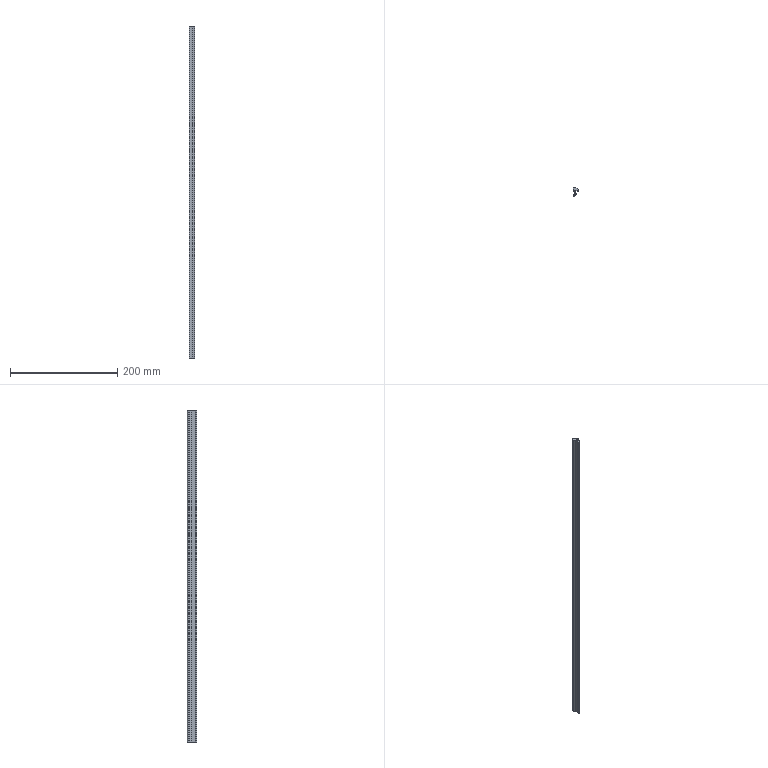Part | SolidWorks | features BaseBody 1, MoveFace 1 | 1 solid | 20 faces | box 10.8 x 17.5 x 620 mm | volume 48856 mm3 | cylinder 11 | plane 9 | commonest cylinder face diameters 1.6 x2 14 x2 0.4 x1 0.6 x1 0.8 x1 2.6 x1
STEP:
#1=CARTESIAN_POINT('',(-3.236,-11.055,520.));
#2=VERTEX_POINT('',#1);
#3=CARTESIAN_POINT('',(-4.3,-10.3,520.));
#4=VERTEX_POINT('',#3);
#5=CARTESIAN_POINT('',(-3.5,-10.3,520.));
#6=DIRECTION('',(0.,0.,-1.));
#7=DIRECTION('',(1.,0.,0.));
#8=AXIS2_PLACEMENT_3D('',#5,#6,#7);
#9=CIRCLE('',#8,0.8);
#10=EDGE_CURVE('',#2,#4,#9,.T.);
#11=ORIENTED_EDGE('',*,*,#10,.T.);
#12=CARTESIAN_POINT('',(-4.3,-10.3,-100.));
#13=VERTEX_POINT('',#12);
#14=CARTESIAN_POINT('',(-4.3,-10.3,-100.));
#15=DIRECTION('',(0.,0.,-1.));
#16=VECTOR('',#15,1000.);
#17=LINE('',#14,#16);
#18=EDGE_CURVE('',#4,#13,#17,.T.);
#19=ORIENTED_EDGE('',*,*,#18,.T.);
#20=CARTESIAN_POINT('',(-3.236,-11.055,-100.));
#21=VERTEX_POINT('',#20);
#22=CARTESIAN_POINT('',(-3.5,-10.3,-100.));
#23=DIRECTION('',(0.,0.,1.));
#24=DIRECTION('',(-1.,0.,0.));
#25=AXIS2_PLACEMENT_3D('',#22,#23,#24);
#26=CIRCLE('',#25,0.8);
#27=EDGE_CURVE('',#13,#21,#26,.T.);
#28=ORIENTED_EDGE('',*,*,#27,.T.);
#29=CARTESIAN_POINT('',(-3.236,-11.055,-100.));
#30=DIRECTION('',(0.,0.,-1.));
#31=VECTOR('',#30,1000.);
#32=LINE('',#29,#31);
#33=EDGE_CURVE('',#2,#21,#32,.T.);
#34=ORIENTED_EDGE('',*,*,#33,.F.);
#35=EDGE_LOOP('',(#11,#19,#28,#34));
#36=FACE_OUTER_BOUND('',#35,.T.);
#37=CARTESIAN_POINT('',(-3.5,-10.3,-100.));
#38=DIRECTION('',(0.,0.,-1.));
#39=DIRECTION('',(-1.,0.,0.));
#40=AXIS2_PLACEMENT_3D('',#37,#38,#39);
#41=CYLINDRICAL_SURFACE('',#40,0.8);
#42=ADVANCED_FACE('',(#36),#41,.T.);
#43=CARTESIAN_POINT('',(1.184,-6.397,-100.));
#44=VERTEX_POINT('',#43);
#45=CARTESIAN_POINT('',(-5.702,-4.29,-100.));
#46=DIRECTION('',(0.,0.,1.));
#47=DIRECTION('',(-1.,0.,0.));
#48=AXIS2_PLACEMENT_3D('',#45,#46,#47);
#49=CIRCLE('',#48,7.201);
#50=EDGE_CURVE('',#21,#44,#49,.T.);
#51=ORIENTED_EDGE('',*,*,#50,.T.);
#52=CARTESIAN_POINT('',(1.184,-6.397,520.));
#53=VERTEX_POINT('',#52);
#54=CARTESIAN_POINT('',(1.184,-6.397,-100.));
#55=DIRECTION('',(0.,0.,1.));
#56=VECTOR('',#55,1000.);
#57=LINE('',#54,#56);
#58=EDGE_CURVE('',#44,#53,#57,.T.);
#59=ORIENTED_EDGE('',*,*,#58,.T.);
#60=CARTESIAN_POINT('',(-5.702,-4.29,520.));
#61=DIRECTION('',(0.,0.,-1.));
#62=DIRECTION('',(1.,0.,0.));
#63=AXIS2_PLACEMENT_3D('',#60,#61,#62);
#64=CIRCLE('',#63,7.201);
#65=EDGE_CURVE('',#53,#2,#64,.T.);
#66=ORIENTED_EDGE('',*,*,#65,.T.);
#67=ORIENTED_EDGE('',*,*,#33,.T.);
#68=EDGE_LOOP('',(#51,#59,#66,#67));
#69=FACE_OUTER_BOUND('',#68,.T.);
#70=CARTESIAN_POINT('',(-5.702,-4.29,-100.));
#71=DIRECTION('',(0.,0.,-1.));
#72=DIRECTION('',(-1.,0.,0.));
#73=AXIS2_PLACEMENT_3D('',#70,#71,#72);
#74=CYLINDRICAL_SURFACE('',#73,7.201);
#75=ADVANCED_FACE('',(#69),#74,.T.);
#76=CARTESIAN_POINT('',(0.9,-6.,-100.));
#77=VERTEX_POINT('',#76);
#78=CARTESIAN_POINT('',(0.9,-6.3,-100.));
#79=DIRECTION('',(0.,0.,1.));
#80=DIRECTION('',(-1.,0.,0.));
#81=AXIS2_PLACEMENT_3D('',#78,#79,#80);
#82=CIRCLE('',#81,0.3);
#83=EDGE_CURVE('',#44,#77,#82,.T.);
#84=ORIENTED_EDGE('',*,*,#83,.T.);
#85=CARTESIAN_POINT('',(0.9,-6.,520.));
#86=VERTEX_POINT('',#85);
#87=CARTESIAN_POINT('',(0.9,-6.,-100.));
#88=DIRECTION('',(0.,0.,1.));
#89=VECTOR('',#88,1000.);
#90=LINE('',#87,#89);
#91=EDGE_CURVE('',#77,#86,#90,.T.);
#92=ORIENTED_EDGE('',*,*,#91,.T.);
#93=CARTESIAN_POINT('',(0.9,-6.3,520.));
#94=DIRECTION('',(0.,0.,-1.));
#95=DIRECTION('',(1.,0.,0.));
#96=AXIS2_PLACEMENT_3D('',#93,#94,#95);
#97=CIRCLE('',#96,0.3);
#98=EDGE_CURVE('',#86,#53,#97,.T.);
#99=ORIENTED_EDGE('',*,*,#98,.T.);
#100=ORIENTED_EDGE('',*,*,#58,.F.);
#101=EDGE_LOOP('',(#84,#92,#99,#100));
#102=FACE_OUTER_BOUND('',#101,.T.);
#103=CARTESIAN_POINT('',(0.9,-6.3,-100.));
#104=DIRECTION('',(0.,0.,-1.));
#105=DIRECTION('',(-1.,0.,0.));
#106=AXIS2_PLACEMENT_3D('',#103,#104,#105);
#107=CYLINDRICAL_SURFACE('',#106,0.3);
#108=ADVANCED_FACE('',(#102),#107,.T.);
#109=CARTESIAN_POINT('',(-2.5,-0.5,-100.));
#110=VERTEX_POINT('',#109);
#111=CARTESIAN_POINT('',(-2.5,-6.153,-100.));
#112=VERTEX_POINT('',#111);
#113=CARTESIAN_POINT('',(-2.5,-6.397,-100.));
#114=DIRECTION('',(0.,-1.,0.));
#115=VECTOR('',#114,1000.);
#116=LINE('',#113,#115);
#117=EDGE_CURVE('',#110,#112,#116,.T.);
#118=ORIENTED_EDGE('',*,*,#117,.F.);
#119=CARTESIAN_POINT('',(-4.2,1.695,-100.));
#120=VERTEX_POINT('',#119);
#121=CARTESIAN_POINT('',(-1.701,1.875,-100.));
#122=DIRECTION('',(0.,0.,1.));
#123=DIRECTION('',(-1.,0.,0.));
#124=AXIS2_PLACEMENT_3D('',#121,#122,#123);
#125=CIRCLE('',#124,2.506);
#126=EDGE_CURVE('',#120,#110,#125,.T.);
#127=ORIENTED_EDGE('',*,*,#126,.F.);
#128=CARTESIAN_POINT('',(-4.2,5.1,-100.));
#129=VERTEX_POINT('',#128);
#130=CARTESIAN_POINT('',(-4.2,-6.397,-100.));
#131=DIRECTION('',(0.,-1.,0.));
#132=VECTOR('',#131,1000.);
#133=LINE('',#130,#132);
#134=EDGE_CURVE('',#129,#120,#133,.T.);
#135=ORIENTED_EDGE('',*,*,#134,.F.);
#136=CARTESIAN_POINT('',(-2.892,6.4,-100.));
#137=VERTEX_POINT('',#136);
#138=CARTESIAN_POINT('',(-2.9,5.1,-100.));
#139=DIRECTION('',(0.,0.,1.));
#140=DIRECTION('',(-1.,0.,0.));
#141=AXIS2_PLACEMENT_3D('',#138,#139,#140);
#142=CIRCLE('',#141,1.3);
#143=EDGE_CURVE('',#137,#129,#142,.T.);
#144=ORIENTED_EDGE('',*,*,#143,.F.);
#145=CARTESIAN_POINT('',(0.5,5.5,-100.));
#146=VERTEX_POINT('',#145);
#147=CARTESIAN_POINT('',(-2.934,-0.5999,-100.));
#148=DIRECTION('',(0.,0.,1.));
#149=DIRECTION('',(-1.,0.,0.));
#150=AXIS2_PLACEMENT_3D('',#147,#148,#149);
#151=CIRCLE('',#150,7.);
#152=EDGE_CURVE('',#146,#137,#151,.T.);
#153=ORIENTED_EDGE('',*,*,#152,.F.);
#154=CARTESIAN_POINT('',(5.5,1.7,-100.));
#155=VERTEX_POINT('',#154);
#156=CARTESIAN_POINT('',(5.5,1.7,-100.));
#157=DIRECTION('',(-0.7962,0.6051,0.));
#158=VECTOR('',#157,1000.);
#159=LINE('',#156,#158);
#160=EDGE_CURVE('',#155,#146,#159,.T.);
#161=ORIENTED_EDGE('',*,*,#160,.F.);
#162=CARTESIAN_POINT('',(6.458,-0.2215,-100.));
#163=VERTEX_POINT('',#162);
#164=CARTESIAN_POINT('',(6.458,-0.2215,-100.));
#165=DIRECTION('',(-0.4462,0.8949,0.));
#166=VECTOR('',#165,1000.);
#167=LINE('',#164,#166);
#168=EDGE_CURVE('',#163,#155,#167,.T.);
#169=ORIENTED_EDGE('',*,*,#168,.F.);
#170=CARTESIAN_POINT('',(5.895,-0.7433,-100.));
#171=VERTEX_POINT('',#170);
#172=CARTESIAN_POINT('',(6.1,-0.4,-100.));
#173=DIRECTION('',(0.,0.,1.));
#174=DIRECTION('',(-1.,0.,0.));
#175=AXIS2_PLACEMENT_3D('',#172,#173,#174);
#176=CIRCLE('',#175,0.4);
#177=EDGE_CURVE('',#171,#163,#176,.T.);
#178=ORIENTED_EDGE('',*,*,#177,.F.);
#179=CARTESIAN_POINT('',(3.,0.,-100.));
#180=VERTEX_POINT('',#179);
#181=CARTESIAN_POINT('',(2.746,-6.995,-100.));
#182=DIRECTION('',(0.,0.,-1.));
#183=DIRECTION('',(-1.,0.,0.));
#184=AXIS2_PLACEMENT_3D('',#181,#182,#183);
#185=CIRCLE('',#184,7.);
#186=EDGE_CURVE('',#180,#171,#185,.T.);
#187=ORIENTED_EDGE('',*,*,#186,.F.);
#188=CARTESIAN_POINT('',(0.,0.,-100.));
#189=VERTEX_POINT('',#188);
#190=CARTESIAN_POINT('',(-6.814,0.,-100.));
#191=DIRECTION('',(1.,0.,0.));
#192=VECTOR('',#191,1000.);
#193=LINE('',#190,#192);
#194=EDGE_CURVE('',#189,#180,#193,.T.);
#195=ORIENTED_EDGE('',*,*,#194,.F.);
#196=CARTESIAN_POINT('',(0.,-5.8,-100.));
#197=VERTEX_POINT('',#196);
#198=CARTESIAN_POINT('',(0.,-6.397,-100.));
#199=DIRECTION('',(0.,1.,0.));
#200=VECTOR('',#199,1000.);
#201=LINE('',#198,#200);
#202=EDGE_CURVE('',#197,#189,#201,.T.);
#203=ORIENTED_EDGE('',*,*,#202,.F.);
#204=CARTESIAN_POINT('',(0.2,-6.,-100.));
#205=VERTEX_POINT('',#204);
#206=CARTESIAN_POINT('',(0.2,-5.8,-100.));
#207=DIRECTION('',(0.,0.,1.));
#208=DIRECTION('',(-1.,0.,0.));
#209=AXIS2_PLACEMENT_3D('',#206,#207,#208);
#210=CIRCLE('',#209,0.2);
#211=EDGE_CURVE('',#197,#205,#210,.T.);
#212=ORIENTED_EDGE('',*,*,#211,.T.);
#213=CARTESIAN_POINT('',(-6.814,-6.,-100.));
#214=DIRECTION('',(-1.,0.,0.));
#215=VECTOR('',#214,1000.);
#216=LINE('',#213,#215);
#217=EDGE_CURVE('',#77,#205,#216,.T.);
#218=ORIENTED_EDGE('',*,*,#217,.F.);
#219=ORIENTED_EDGE('',*,*,#83,.F.);
#220=ORIENTED_EDGE('',*,*,#50,.F.);
#221=ORIENTED_EDGE('',*,*,#27,.F.);
#222=CARTESIAN_POINT('',(-3.998,-9.674,-100.));
#223=VERTEX_POINT('',#222);
#224=CARTESIAN_POINT('',(-3.5,-10.3,-100.));
#225=DIRECTION('',(0.,0.,1.));
#226=DIRECTION('',(-1.,0.,0.));
#227=AXIS2_PLACEMENT_3D('',#224,#225,#226);
#228=CIRCLE('',#227,0.8);
#229=EDGE_CURVE('',#223,#13,#228,.T.);
#230=ORIENTED_EDGE('',*,*,#229,.F.);
#231=CARTESIAN_POINT('',(-6.814,-6.397,-100.));
#232=DIRECTION('',(0.,0.,-1.));
#233=DIRECTION('',(-1.,0.,0.));
#234=AXIS2_PLACEMENT_3D('',#231,#232,#233);
#235=CIRCLE('',#234,4.321);
#236=EDGE_CURVE('',#112,#223,#235,.T.);
#237=ORIENTED_EDGE('',*,*,#236,.F.);
#238=EDGE_LOOP('',(#118,#127,#135,#144,#153,#161,#169,#178,#187,#195,#203,#212,#218,#219,#220,#221,#230,#237));
#239=FACE_OUTER_BOUND('',#238,.T.);
#240=CARTESIAN_POINT('',(-6.814,-6.397,-100.));
#241=DIRECTION('',(0.,0.,1.));
#242=DIRECTION('',(1.,0.,0.));
#243=AXIS2_PLACEMENT_3D('',#240,#241,#242);
#244=PLANE('',#243);
#245=ADVANCED_FACE('',(#239),#244,.F.);
#246=ORIENTED_EDGE('',*,*,#18,.F.);
#247=CARTESIAN_POINT('',(-3.998,-9.674,520.));
#248=VERTEX_POINT('',#247);
#249=CARTESIAN_POINT('',(-3.5,-10.3,520.));
#250=DIRECTION('',(0.,0.,-1.));
#251=DIRECTION('',(1.,0.,0.));
#252=AXIS2_PLACEMENT_3D('',#249,#250,#251);
#253=CIRCLE('',#252,0.8);
#254=EDGE_CURVE('',#4,#248,#253,.T.);
#255=ORIENTED_EDGE('',*,*,#254,.T.);
#256=CARTESIAN_POINT('',(-3.998,-9.674,-100.));
#257=DIRECTION('',(0.,0.,-1.));
#258=VECTOR('',#257,1000.);
#259=LINE('',#256,#258);
#260=EDGE_CURVE('',#248,#223,#259,.T.);
#261=ORIENTED_EDGE('',*,*,#260,.T.);
#262=ORIENTED_EDGE('',*,*,#229,.T.);
#263=EDGE_LOOP('',(#246,#255,#261,#262));
#264=FACE_OUTER_BOUND('',#263,.T.);
#265=CARTESIAN_POINT('',(-3.5,-10.3,-100.));
#266=DIRECTION('',(0.,0.,-1.));
#267=DIRECTION('',(-1.,0.,0.));
#268=AXIS2_PLACEMENT_3D('',#265,#266,#267);
#269=CYLINDRICAL_SURFACE('',#268,0.8);
#270=ADVANCED_FACE('',(#264),#269,.T.);
#271=CARTESIAN_POINT('',(-4.2,1.695,520.));
#272=VERTEX_POINT('',#271);
#273=CARTESIAN_POINT('',(-2.5,-0.5,520.));
#274=VERTEX_POINT('',#273);
#275=CARTESIAN_POINT('',(-1.701,1.875,520.));
#276=DIRECTION('',(0.,0.,1.));
#277=DIRECTION('',(1.,0.,0.));
#278=AXIS2_PLACEMENT_3D('',#275,#276,#277);
#279=CIRCLE('',#278,2.506);
#280=EDGE_CURVE('',#272,#274,#279,.T.);
#281=ORIENTED_EDGE('',*,*,#280,.T.);
#282=CARTESIAN_POINT('',(-2.5,-6.153,520.));
#283=VERTEX_POINT('',#282);
#284=CARTESIAN_POINT('',(-2.5,-6.397,520.));
#285=DIRECTION('',(0.,-1.,0.));
#286=VECTOR('',#285,1000.);
#287=LINE('',#284,#286);
#288=EDGE_CURVE('',#274,#283,#287,.T.);
#289=ORIENTED_EDGE('',*,*,#288,.T.);
#290=CARTESIAN_POINT('',(-6.814,-6.397,520.));
#291=DIRECTION('',(0.,0.,-1.));
#292=DIRECTION('',(1.,0.,0.));
#293=AXIS2_PLACEMENT_3D('',#290,#291,#292);
#294=CIRCLE('',#293,4.321);
#295=EDGE_CURVE('',#283,#248,#294,.T.);
#296=ORIENTED_EDGE('',*,*,#295,.T.);
#297=ORIENTED_EDGE('',*,*,#254,.F.);
#298=ORIENTED_EDGE('',*,*,#10,.F.);
#299=ORIENTED_EDGE('',*,*,#65,.F.);
#300=ORIENTED_EDGE('',*,*,#98,.F.);
#301=CARTESIAN_POINT('',(0.2,-6.,520.));
#302=VERTEX_POINT('',#301);
#303=CARTESIAN_POINT('',(-6.814,-6.,520.));
#304=DIRECTION('',(-1.,0.,0.));
#305=VECTOR('',#304,1000.);
#306=LINE('',#303,#305);
#307=EDGE_CURVE('',#86,#302,#306,.T.);
#308=ORIENTED_EDGE('',*,*,#307,.T.);
#309=CARTESIAN_POINT('',(0.,-5.8,520.));
#310=VERTEX_POINT('',#309);
#311=CARTESIAN_POINT('',(0.2,-5.8,520.));
#312=DIRECTION('',(0.,0.,-1.));
#313=DIRECTION('',(1.,0.,0.));
#314=AXIS2_PLACEMENT_3D('',#311,#312,#313);
#315=CIRCLE('',#314,0.2);
#316=EDGE_CURVE('',#302,#310,#315,.T.);
#317=ORIENTED_EDGE('',*,*,#316,.T.);
#318=CARTESIAN_POINT('',(0.,0.,520.));
#319=VERTEX_POINT('',#318);
#320=CARTESIAN_POINT('',(0.,-6.397,520.));
#321=DIRECTION('',(0.,1.,0.));
#322=VECTOR('',#321,1000.);
#323=LINE('',#320,#322);
#324=EDGE_CURVE('',#310,#319,#323,.T.);
#325=ORIENTED_EDGE('',*,*,#324,.T.);
#326=CARTESIAN_POINT('',(3.,0.,520.));
#327=VERTEX_POINT('',#326);
#328=CARTESIAN_POINT('',(-6.814,0.,520.));
#329=DIRECTION('',(1.,0.,0.));
#330=VECTOR('',#329,1000.);
#331=LINE('',#328,#330);
#332=EDGE_CURVE('',#319,#327,#331,.T.);
#333=ORIENTED_EDGE('',*,*,#332,.T.);
#334=CARTESIAN_POINT('',(5.895,-0.7433,520.));
#335=VERTEX_POINT('',#334);
#336=CARTESIAN_POINT('',(2.746,-6.995,520.));
#337=DIRECTION('',(0.,0.,-1.));
#338=DIRECTION('',(1.,0.,0.));
#339=AXIS2_PLACEMENT_3D('',#336,#337,#338);
#340=CIRCLE('',#339,7.);
#341=EDGE_CURVE('',#327,#335,#340,.T.);
#342=ORIENTED_EDGE('',*,*,#341,.T.);
#343=CARTESIAN_POINT('',(6.458,-0.2215,520.));
#344=VERTEX_POINT('',#343);
#345=CARTESIAN_POINT('',(6.1,-0.4,520.));
#346=DIRECTION('',(0.,0.,-1.));
#347=DIRECTION('',(1.,0.,0.));
#348=AXIS2_PLACEMENT_3D('',#345,#346,#347);
#349=CIRCLE('',#348,0.4);
#350=EDGE_CURVE('',#344,#335,#349,.T.);
#351=ORIENTED_EDGE('',*,*,#350,.F.);
#352=CARTESIAN_POINT('',(5.5,1.7,520.));
#353=VERTEX_POINT('',#352);
#354=CARTESIAN_POINT('',(6.282,0.1323,520.));
#355=DIRECTION('',(-0.4462,0.8949,0.));
#356=VECTOR('',#355,1000.);
#357=LINE('',#354,#356);
#358=EDGE_CURVE('',#344,#353,#357,.T.);
#359=ORIENTED_EDGE('',*,*,#358,.T.);
#360=CARTESIAN_POINT('',(0.5,5.5,520.));
#361=VERTEX_POINT('',#360);
#362=CARTESIAN_POINT('',(1.595,4.668,520.));
#363=DIRECTION('',(-0.7962,0.6051,0.));
#364=VECTOR('',#363,1000.);
#365=LINE('',#362,#364);
#366=EDGE_CURVE('',#353,#361,#365,.T.);
#367=ORIENTED_EDGE('',*,*,#366,.T.);
#368=CARTESIAN_POINT('',(-2.892,6.4,520.));
#369=VERTEX_POINT('',#368);
#370=CARTESIAN_POINT('',(-2.934,-0.5999,520.));
#371=DIRECTION('',(0.,0.,1.));
#372=DIRECTION('',(1.,0.,0.));
#373=AXIS2_PLACEMENT_3D('',#370,#371,#372);
#374=CIRCLE('',#373,7.);
#375=EDGE_CURVE('',#361,#369,#374,.T.);
#376=ORIENTED_EDGE('',*,*,#375,.T.);
#377=CARTESIAN_POINT('',(-4.2,5.1,520.));
#378=VERTEX_POINT('',#377);
#379=CARTESIAN_POINT('',(-2.9,5.1,520.));
#380=DIRECTION('',(0.,0.,1.));
#381=DIRECTION('',(1.,0.,0.));
#382=AXIS2_PLACEMENT_3D('',#379,#380,#381);
#383=CIRCLE('',#382,1.3);
#384=EDGE_CURVE('',#369,#378,#383,.T.);
#385=ORIENTED_EDGE('',*,*,#384,.T.);
#386=CARTESIAN_POINT('',(-4.2,-6.397,520.));
#387=DIRECTION('',(0.,-1.,0.));
#388=VECTOR('',#387,1000.);
#389=LINE('',#386,#388);
#390=EDGE_CURVE('',#378,#272,#389,.T.);
#391=ORIENTED_EDGE('',*,*,#390,.T.);
#392=EDGE_LOOP('',(#281,#289,#296,#297,#298,#299,#300,#308,#317,#325,#333,#342,#351,#359,#367,#376,#385,#391));
#393=FACE_OUTER_BOUND('',#392,.T.);
#394=CARTESIAN_POINT('',(-6.814,-6.397,520.));
#395=DIRECTION('',(0.,0.,1.));
#396=DIRECTION('',(1.,0.,0.));
#397=AXIS2_PLACEMENT_3D('',#394,#395,#396);
#398=PLANE('',#397);
#399=ADVANCED_FACE('',(#393),#398,.T.);
#400=ORIENTED_EDGE('',*,*,#217,.T.);
#401=CARTESIAN_POINT('',(0.2,-6.,-100.));
#402=DIRECTION('',(0.,0.,1.));
#403=VECTOR('',#402,1000.);
#404=LINE('',#401,#403);
#405=EDGE_CURVE('',#205,#302,#404,.T.);
#406=ORIENTED_EDGE('',*,*,#405,.T.);
#407=ORIENTED_EDGE('',*,*,#307,.F.);
#408=ORIENTED_EDGE('',*,*,#91,.F.);
#409=EDGE_LOOP('',(#400,#406,#407,#408));
#410=FACE_OUTER_BOUND('',#409,.T.);
#411=CARTESIAN_POINT('',(0.9,-6.,-100.));
#412=DIRECTION('',(0.,1.,0.));
#413=DIRECTION('',(0.,0.,1.));
#414=AXIS2_PLACEMENT_3D('',#411,#412,#413);
#415=PLANE('',#414);
#416=ADVANCED_FACE('',(#410),#415,.T.);
#417=CARTESIAN_POINT('',(-2.5,-6.153,-100.));
#418=DIRECTION('',(0.,0.,1.));
#419=VECTOR('',#418,1000.);
#420=LINE('',#417,#419);
#421=EDGE_CURVE('',#112,#283,#420,.T.);
#422=ORIENTED_EDGE('',*,*,#421,.F.);
#423=ORIENTED_EDGE('',*,*,#236,.T.);
#424=ORIENTED_EDGE('',*,*,#260,.F.);
#425=ORIENTED_EDGE('',*,*,#295,.F.);
#426=EDGE_LOOP('',(#422,#423,#424,#425));
#427=FACE_OUTER_BOUND('',#426,.T.);
#428=CARTESIAN_POINT('',(-6.814,-6.397,-100.));
#429=DIRECTION('',(0.,0.,-1.));
#430=DIRECTION('',(-1.,0.,0.));
#431=AXIS2_PLACEMENT_3D('',#428,#429,#430);
#432=CYLINDRICAL_SURFACE('',#431,4.321);
#433=ADVANCED_FACE('',(#427),#432,.F.);
#434=ORIENTED_EDGE('',*,*,#117,.T.);
#435=ORIENTED_EDGE('',*,*,#421,.T.);
#436=ORIENTED_EDGE('',*,*,#288,.F.);
#437=CARTESIAN_POINT('',(-2.5,-0.5,-100.));
#438=DIRECTION('',(0.,0.,-1.));
#439=VECTOR('',#438,1000.);
#440=LINE('',#437,#439);
#441=EDGE_CURVE('',#274,#110,#440,.T.);
#442=ORIENTED_EDGE('',*,*,#441,.T.);
#443=EDGE_LOOP('',(#434,#435,#436,#442));
#444=FACE_OUTER_BOUND('',#443,.T.);
#445=CARTESIAN_POINT('',(-2.5,-0.5,-100.));
#446=DIRECTION('',(-1.,0.,0.));
#447=DIRECTION('',(0.,0.,1.));
#448=AXIS2_PLACEMENT_3D('',#445,#446,#447);
#449=PLANE('',#448);
#450=ADVANCED_FACE('',(#444),#449,.T.);
#451=ORIENTED_EDGE('',*,*,#126,.T.);
#452=ORIENTED_EDGE('',*,*,#441,.F.);
#453=ORIENTED_EDGE('',*,*,#280,.F.);
#454=CARTESIAN_POINT('',(-4.2,1.695,-100.));
#455=DIRECTION('',(0.,0.,-1.));
#456=VECTOR('',#455,1000.);
#457=LINE('',#454,#456);
#458=EDGE_CURVE('',#272,#120,#457,.T.);
#459=ORIENTED_EDGE('',*,*,#458,.T.);
#460=EDGE_LOOP('',(#451,#452,#453,#459));
#461=FACE_OUTER_BOUND('',#460,.T.);
#462=CARTESIAN_POINT('',(-1.701,1.875,-100.));
#463=DIRECTION('',(0.,0.,-1.));
#464=DIRECTION('',(-1.,0.,0.));
#465=AXIS2_PLACEMENT_3D('',#462,#463,#464);
#466=CYLINDRICAL_SURFACE('',#465,2.506);
#467=ADVANCED_FACE('',(#461),#466,.T.);
#468=ORIENTED_EDGE('',*,*,#134,.T.);
#469=ORIENTED_EDGE('',*,*,#458,.F.);
#470=ORIENTED_EDGE('',*,*,#390,.F.);
#471=CARTESIAN_POINT('',(-4.2,5.1,-100.));
#472=DIRECTION('',(0.,0.,-1.));
#473=VECTOR('',#472,1000.);
#474=LINE('',#471,#473);
#475=EDGE_CURVE('',#378,#129,#474,.T.);
#476=ORIENTED_EDGE('',*,*,#475,.T.);
#477=EDGE_LOOP('',(#468,#469,#470,#476));
#478=FACE_OUTER_BOUND('',#477,.T.);
#479=CARTESIAN_POINT('',(-4.2,5.1,-100.));
#480=DIRECTION('',(-1.,0.,0.));
#481=DIRECTION('',(0.,0.,1.));
#482=AXIS2_PLACEMENT_3D('',#479,#480,#481);
#483=PLANE('',#482);
#484=ADVANCED_FACE('',(#478),#483,.T.);
#485=ORIENTED_EDGE('',*,*,#143,.T.);
#486=ORIENTED_EDGE('',*,*,#475,.F.);
#487=ORIENTED_EDGE('',*,*,#384,.F.);
#488=CARTESIAN_POINT('',(-2.892,6.4,-100.));
#489=DIRECTION('',(0.,0.,-1.));
#490=VECTOR('',#489,1000.);
#491=LINE('',#488,#490);
#492=EDGE_CURVE('',#369,#137,#491,.T.);
#493=ORIENTED_EDGE('',*,*,#492,.T.);
#494=EDGE_LOOP('',(#485,#486,#487,#493));
#495=FACE_OUTER_BOUND('',#494,.T.);
#496=CARTESIAN_POINT('',(-2.9,5.1,-100.));
#497=DIRECTION('',(0.,0.,-1.));
#498=DIRECTION('',(-1.,0.,0.));
#499=AXIS2_PLACEMENT_3D('',#496,#497,#498);
#500=CYLINDRICAL_SURFACE('',#499,1.3);
#501=ADVANCED_FACE('',(#495),#500,.T.);
#502=ORIENTED_EDGE('',*,*,#152,.T.);
#503=ORIENTED_EDGE('',*,*,#492,.F.);
#504=ORIENTED_EDGE('',*,*,#375,.F.);
#505=CARTESIAN_POINT('',(0.5,5.5,-100.));
#506=DIRECTION('',(0.,0.,-1.));
#507=VECTOR('',#506,1000.);
#508=LINE('',#505,#507);
#509=EDGE_CURVE('',#361,#146,#508,.T.);
#510=ORIENTED_EDGE('',*,*,#509,.T.);
#511=EDGE_LOOP('',(#502,#503,#504,#510));
#512=FACE_OUTER_BOUND('',#511,.T.);
#513=CARTESIAN_POINT('',(-2.934,-0.5999,-100.));
#514=DIRECTION('',(0.,0.,-1.));
#515=DIRECTION('',(-1.,0.,0.));
#516=AXIS2_PLACEMENT_3D('',#513,#514,#515);
#517=CYLINDRICAL_SURFACE('',#516,7.);
#518=ADVANCED_FACE('',(#512),#517,.T.);
#519=ORIENTED_EDGE('',*,*,#160,.T.);
#520=ORIENTED_EDGE('',*,*,#509,.F.);
#521=ORIENTED_EDGE('',*,*,#366,.F.);
#522=CARTESIAN_POINT('',(5.5,1.7,-100.));
#523=DIRECTION('',(0.,0.,-1.));
#524=VECTOR('',#523,1000.);
#525=LINE('',#522,#524);
#526=EDGE_CURVE('',#353,#155,#525,.T.);
#527=ORIENTED_EDGE('',*,*,#526,.T.);
#528=EDGE_LOOP('',(#519,#520,#521,#527));
#529=FACE_OUTER_BOUND('',#528,.T.);
#530=CARTESIAN_POINT('',(5.5,1.7,-100.));
#531=DIRECTION('',(0.6051,0.7962,0.));
#532=DIRECTION('',(-0.7962,0.6051,0.));
#533=AXIS2_PLACEMENT_3D('',#530,#531,#532);
#534=PLANE('',#533);
#535=ADVANCED_FACE('',(#529),#534,.T.);
#536=ORIENTED_EDGE('',*,*,#168,.T.);
#537=ORIENTED_EDGE('',*,*,#526,.F.);
#538=ORIENTED_EDGE('',*,*,#358,.F.);
#539=CARTESIAN_POINT('',(6.458,-0.2215,-100.));
#540=DIRECTION('',(0.,0.,-1.));
#541=VECTOR('',#540,1000.);
#542=LINE('',#539,#541);
#543=EDGE_CURVE('',#344,#163,#542,.T.);
#544=ORIENTED_EDGE('',*,*,#543,.T.);
#545=EDGE_LOOP('',(#536,#537,#538,#544));
#546=FACE_OUTER_BOUND('',#545,.T.);
#547=CARTESIAN_POINT('',(6.458,-0.2215,-100.));
#548=DIRECTION('',(0.8949,0.4462,0.));
#549=DIRECTION('',(-0.4462,0.8949,0.));
#550=AXIS2_PLACEMENT_3D('',#547,#548,#549);
#551=PLANE('',#550);
#552=ADVANCED_FACE('',(#546),#551,.T.);
#553=CARTESIAN_POINT('',(3.,0.,-100.));
#554=DIRECTION('',(0.,0.,1.));
#555=VECTOR('',#554,1000.);
#556=LINE('',#553,#555);
#557=EDGE_CURVE('',#180,#327,#556,.T.);
#558=ORIENTED_EDGE('',*,*,#557,.F.);
#559=ORIENTED_EDGE('',*,*,#186,.T.);
#560=CARTESIAN_POINT('',(5.895,-0.7433,-100.));
#561=DIRECTION('',(0.,0.,-1.));
#562=VECTOR('',#561,1000.);
#563=LINE('',#560,#562);
#564=EDGE_CURVE('',#335,#171,#563,.T.);
#565=ORIENTED_EDGE('',*,*,#564,.F.);
#566=ORIENTED_EDGE('',*,*,#341,.F.);
#567=EDGE_LOOP('',(#558,#559,#565,#566));
#568=FACE_OUTER_BOUND('',#567,.T.);
#569=CARTESIAN_POINT('',(2.746,-6.995,-100.));
#570=DIRECTION('',(0.,0.,-1.));
#571=DIRECTION('',(-1.,0.,0.));
#572=AXIS2_PLACEMENT_3D('',#569,#570,#571);
#573=CYLINDRICAL_SURFACE('',#572,7.);
#574=ADVANCED_FACE('',(#568),#573,.F.);
#575=ORIENTED_EDGE('',*,*,#194,.T.);
#576=ORIENTED_EDGE('',*,*,#557,.T.);
#577=ORIENTED_EDGE('',*,*,#332,.F.);
#578=CARTESIAN_POINT('',(0.,0.,-100.));
#579=DIRECTION('',(0.,0.,-1.));
#580=VECTOR('',#579,1000.);
#581=LINE('',#578,#580);
#582=EDGE_CURVE('',#319,#189,#581,.T.);
#583=ORIENTED_EDGE('',*,*,#582,.T.);
#584=EDGE_LOOP('',(#575,#576,#577,#583));
#585=FACE_OUTER_BOUND('',#584,.T.);
#586=CARTESIAN_POINT('',(0.,0.,-100.));
#587=DIRECTION('',(0.,-1.,0.));
#588=DIRECTION('',(0.,0.,-1.));
#589=AXIS2_PLACEMENT_3D('',#586,#587,#588);
#590=PLANE('',#589);
#591=ADVANCED_FACE('',(#585),#590,.T.);
#592=ORIENTED_EDGE('',*,*,#202,.T.);
#593=ORIENTED_EDGE('',*,*,#582,.F.);
#594=ORIENTED_EDGE('',*,*,#324,.F.);
#595=CARTESIAN_POINT('',(0.,-5.8,-100.));
#596=DIRECTION('',(0.,0.,-1.));
#597=VECTOR('',#596,1000.);
#598=LINE('',#595,#597);
#599=EDGE_CURVE('',#310,#197,#598,.T.);
#600=ORIENTED_EDGE('',*,*,#599,.T.);
#601=EDGE_LOOP('',(#592,#593,#594,#600));
#602=FACE_OUTER_BOUND('',#601,.T.);
#603=CARTESIAN_POINT('',(0.,-5.8,-100.));
#604=DIRECTION('',(1.,0.,0.));
#605=DIRECTION('',(0.,0.,-1.));
#606=AXIS2_PLACEMENT_3D('',#603,#604,#605);
#607=PLANE('',#606);
#608=ADVANCED_FACE('',(#602),#607,.T.);
#609=ORIENTED_EDGE('',*,*,#405,.F.);
#610=ORIENTED_EDGE('',*,*,#211,.F.);
#611=ORIENTED_EDGE('',*,*,#599,.F.);
#612=ORIENTED_EDGE('',*,*,#316,.F.);
#613=EDGE_LOOP('',(#609,#610,#611,#612));
#614=FACE_OUTER_BOUND('',#613,.T.);
#615=CARTESIAN_POINT('',(0.2,-5.8,-100.));
#616=DIRECTION('',(0.,0.,-1.));
#617=DIRECTION('',(-1.,0.,0.));
#618=AXIS2_PLACEMENT_3D('',#615,#616,#617);
#619=CYLINDRICAL_SURFACE('',#618,0.2);
#620=ADVANCED_FACE('',(#614),#619,.F.);
#621=ORIENTED_EDGE('',*,*,#177,.T.);
#622=ORIENTED_EDGE('',*,*,#543,.F.);
#623=ORIENTED_EDGE('',*,*,#350,.T.);
#624=ORIENTED_EDGE('',*,*,#564,.T.);
#625=EDGE_LOOP('',(#621,#622,#623,#624));
#626=FACE_OUTER_BOUND('',#625,.T.);
#627=CARTESIAN_POINT('',(6.1,-0.4,-100.));
#628=DIRECTION('',(0.,0.,-1.));
#629=DIRECTION('',(-1.,0.,0.));
#630=AXIS2_PLACEMENT_3D('',#627,#628,#629);
#631=CYLINDRICAL_SURFACE('',#630,0.4);
#632=ADVANCED_FACE('',(#626),#631,.T.);
#633=CLOSED_SHELL('',(#42,#75,#108,#245,#270,#399,#416,#433,#450,#467,#484,#501,#518,#535,#552,#574,#591,#608,#620,#632));
#634=MANIFOLD_SOLID_BREP('',#633);
#635=CARTESIAN_POINT('',(0.,0.,0.));
#636=DIRECTION('',(0.,0.,1.));
#637=DIRECTION('',(1.,0.,0.));
#638=AXIS2_PLACEMENT_3D('',#635,#636,#637);
#639=(LENGTH_UNIT()NAMED_UNIT(*)SI_UNIT(.MILLI.,.METRE.));
#640=UNCERTAINTY_MEASURE_WITH_UNIT(LENGTH_MEASURE(0.00001),#639,'','');
#641=(NAMED_UNIT(*)PLANE_ANGLE_UNIT()SI_UNIT($,.RADIAN.));
#642=(NAMED_UNIT(*)SI_UNIT($,.STERADIAN.)SOLID_ANGLE_UNIT());
#643=(GEOMETRIC_REPRESENTATION_CONTEXT(3)GLOBAL_UNCERTAINTY_ASSIGNED_CONTEXT((#640))GLOBAL_UNIT_ASSIGNED_CONTEXT((#639,#641,#642))REPRESENTATION_CONTEXT('',''));
#644=ADVANCED_BREP_SHAPE_REPRESENTATION('',(#634,#638),#643);